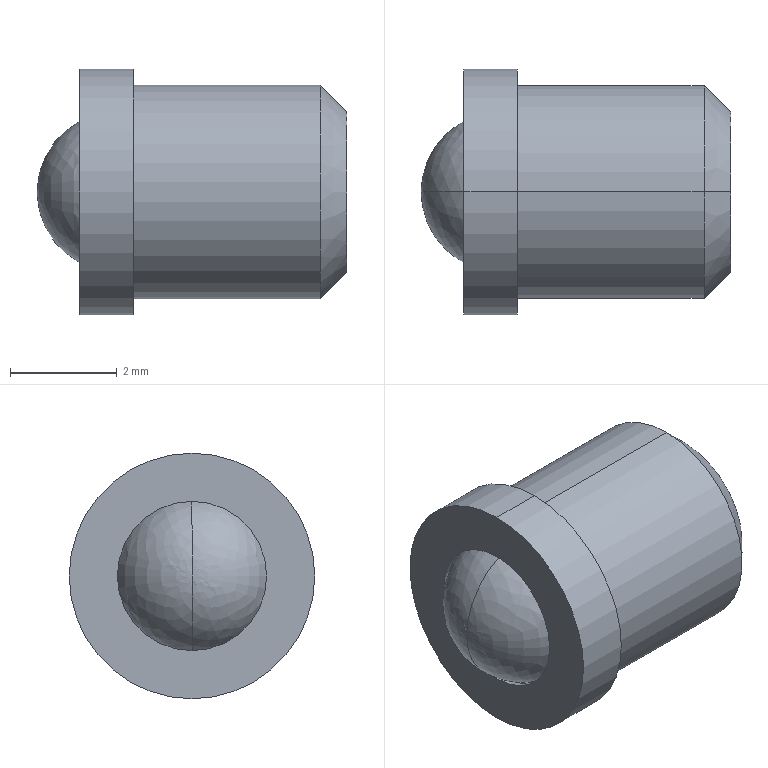Part | SolidWorks | features BaseBody 1 | 1 solid | 16 faces | box 5.8 x 4.6 x 4.6 mm | volume 67.656 mm3 | cylinder 8 | plane 4 | spline 2 | cone 2 | commonest cylinder face diameters 2.8 x2 3 x2 4 x2 4.6 x2
STEP:
#1=CARTESIAN_POINT('',(484.737,37.715,65.366));
#2=VERTEX_POINT('',#1);
#3=CARTESIAN_POINT('',(486.237,37.715,63.866));
#4=VERTEX_POINT('',#3);
#5=CARTESIAN_POINT('',(484.737,37.715,65.366));
#6=CARTESIAN_POINT('',(484.737,37.715,65.266));
#7=CARTESIAN_POINT('',(484.757,37.715,65.066));
#8=CARTESIAN_POINT('',(484.846,37.715,64.777));
#9=CARTESIAN_POINT('',(484.991,37.715,64.512));
#10=CARTESIAN_POINT('',(485.186,37.715,64.282));
#11=CARTESIAN_POINT('',(485.423,37.715,64.094));
#12=CARTESIAN_POINT('',(485.692,37.715,63.958));
#13=CARTESIAN_POINT('',(485.968,37.715,63.882));
#14=CARTESIAN_POINT('',(486.152,37.715,63.866));
#15=CARTESIAN_POINT('',(486.237,37.715,63.866));
#16=B_SPLINE_CURVE_WITH_KNOTS('',3,(#5,#6,#7,#8,#9,#10,#11,#12,#13,#14,#15),.UNSPECIFIED.,.F.,.F.,(4,1,1,1,1,1,1,1,4),(0.,0.125,0.25,0.375,0.5,0.625,0.75,0.875,0.9804),.UNSPECIFIED.);
#17=EDGE_CURVE('',#2,#4,#16,.T.);
#18=ORIENTED_EDGE('',*,*,#17,.F.);
#19=CARTESIAN_POINT('',(486.237,37.715,66.866));
#20=VERTEX_POINT('',#19);
#21=CARTESIAN_POINT('',(484.737,37.715,65.366));
#22=CARTESIAN_POINT('',(484.737,37.715,65.466));
#23=CARTESIAN_POINT('',(484.757,37.715,65.666));
#24=CARTESIAN_POINT('',(484.846,37.715,65.955));
#25=CARTESIAN_POINT('',(484.991,37.715,66.22));
#26=CARTESIAN_POINT('',(485.186,37.715,66.45));
#27=CARTESIAN_POINT('',(485.423,37.715,66.638));
#28=CARTESIAN_POINT('',(485.692,37.715,66.774));
#29=CARTESIAN_POINT('',(485.968,37.715,66.85));
#30=CARTESIAN_POINT('',(486.152,37.715,66.866));
#31=CARTESIAN_POINT('',(486.237,37.715,66.866));
#32=B_SPLINE_CURVE_WITH_KNOTS('',3,(#21,#22,#23,#24,#25,#26,#27,#28,#29,#30,#31),.UNSPECIFIED.,.F.,.F.,(4,1,1,1,1,1,1,1,4),(0.,0.125,0.25,0.375,0.5,0.625,0.75,0.875,0.9804),.UNSPECIFIED.);
#33=EDGE_CURVE('',#2,#20,#32,.T.);
#34=ORIENTED_EDGE('',*,*,#33,.T.);
#35=CARTESIAN_POINT('',(486.237,37.715,65.366));
#36=DIRECTION('',(1.,0.,0.000000013));
#37=DIRECTION('',(0.000000013,0.,-1.));
#38=AXIS2_PLACEMENT_3D('',#35,#36,#37);
#39=CIRCLE('',#38,1.5);
#40=EDGE_CURVE('',#4,#20,#39,.T.);
#41=ORIENTED_EDGE('',*,*,#40,.F.);
#42=EDGE_LOOP('',(#18,#34,#41));
#43=FACE_OUTER_BOUND('',#42,.T.);
#44=CARTESIAN_POINT('',(484.737,37.715,65.366));
#45=CARTESIAN_POINT('',(484.737,37.715,65.366));
#46=CARTESIAN_POINT('',(484.737,37.715,65.366));
#47=CARTESIAN_POINT('',(484.737,37.715,65.366));
#48=CARTESIAN_POINT('',(484.737,37.715,65.266));
#49=CARTESIAN_POINT('',(484.737,37.915,65.266));
#50=CARTESIAN_POINT('',(484.737,37.915,65.466));
#51=CARTESIAN_POINT('',(484.737,37.715,65.466));
#52=CARTESIAN_POINT('',(484.757,37.715,65.066));
#53=CARTESIAN_POINT('',(484.757,38.316,65.066));
#54=CARTESIAN_POINT('',(484.757,38.316,65.666));
#55=CARTESIAN_POINT('',(484.757,37.715,65.666));
#56=CARTESIAN_POINT('',(484.846,37.715,64.777));
#57=CARTESIAN_POINT('',(484.846,38.892,64.777));
#58=CARTESIAN_POINT('',(484.846,38.892,65.955));
#59=CARTESIAN_POINT('',(484.846,37.715,65.955));
#60=CARTESIAN_POINT('',(484.991,37.715,64.512));
#61=CARTESIAN_POINT('',(484.991,39.422,64.512));
#62=CARTESIAN_POINT('',(484.991,39.422,66.22));
#63=CARTESIAN_POINT('',(484.991,37.715,66.22));
#64=CARTESIAN_POINT('',(485.186,37.715,64.282));
#65=CARTESIAN_POINT('',(485.186,39.884,64.282));
#66=CARTESIAN_POINT('',(485.186,39.884,66.45));
#67=CARTESIAN_POINT('',(485.186,37.715,66.45));
#68=CARTESIAN_POINT('',(485.423,37.715,64.094));
#69=CARTESIAN_POINT('',(485.423,40.258,64.094));
#70=CARTESIAN_POINT('',(485.423,40.258,66.638));
#71=CARTESIAN_POINT('',(485.423,37.715,66.638));
#72=CARTESIAN_POINT('',(485.692,37.715,63.958));
#73=CARTESIAN_POINT('',(485.692,40.531,63.958));
#74=CARTESIAN_POINT('',(485.692,40.531,66.774));
#75=CARTESIAN_POINT('',(485.692,37.715,66.774));
#76=CARTESIAN_POINT('',(485.968,37.715,63.882));
#77=CARTESIAN_POINT('',(485.968,40.683,63.882));
#78=CARTESIAN_POINT('',(485.968,40.683,66.85));
#79=CARTESIAN_POINT('',(485.968,37.715,66.85));
#80=CARTESIAN_POINT('',(486.152,37.715,63.866));
#81=CARTESIAN_POINT('',(486.152,40.715,63.866));
#82=CARTESIAN_POINT('',(486.152,40.715,66.866));
#83=CARTESIAN_POINT('',(486.152,37.715,66.866));
#84=CARTESIAN_POINT('',(486.237,37.715,63.866));
#85=CARTESIAN_POINT('',(486.237,40.715,63.866));
#86=CARTESIAN_POINT('',(486.237,40.715,66.866));
#87=CARTESIAN_POINT('',(486.237,37.715,66.866));
#88=(BOUNDED_SURFACE()B_SPLINE_SURFACE(3,3,((#44,#45,#46,#47),(#48,#49,#50,#51),(#52,#53,#54,#55),(#56,#57,#58,#59),(#60,#61,#62,#63),(#64,#65,#66,#67),(#68,#69,#70,#71),(#72,#73,#74,#75),(#76,#77,#78,#79),(#80,#81,#82,#83),(#84,#85,#86,#87)),.UNSPECIFIED.,.F.,.F.,.F.)B_SPLINE_SURFACE_WITH_KNOTS((4,1,1,1,1,1,1,1,4),(4,4),(0.,0.125,0.25,0.375,0.5,0.625,0.75,0.875,0.9804),(0.,1.),.UNSPECIFIED.)GEOMETRIC_REPRESENTATION_ITEM()RATIONAL_B_SPLINE_SURFACE(((1.,0.3333,0.3333,1.),(1.,0.3333,0.3333,1.),(1.,0.3333,0.3333,1.),(1.,0.3333,0.3333,1.),(1.,0.3333,0.3333,1.),(1.,0.3333,0.3333,1.),(1.,0.3333,0.3333,1.),(1.,0.3333,0.3333,1.),(1.,0.3333,0.3333,1.),(1.,0.3333,0.3333,1.),(1.,0.3333,0.3333,1.)))REPRESENTATION_ITEM('')SURFACE());
#89=ADVANCED_FACE('',(#43),#88,.F.);
#90=CARTESIAN_POINT('',(486.537,37.715,67.366));
#91=VERTEX_POINT('',#90);
#92=CARTESIAN_POINT('',(486.537,37.715,63.366));
#93=VERTEX_POINT('',#92);
#94=CARTESIAN_POINT('',(486.537,37.715,65.366));
#95=DIRECTION('',(-1.,0.,-0.000000013));
#96=DIRECTION('',(0.000000013,0.,-1.));
#97=AXIS2_PLACEMENT_3D('',#94,#95,#96);
#98=CIRCLE('',#97,2.);
#99=EDGE_CURVE('',#91,#93,#98,.T.);
#100=ORIENTED_EDGE('',*,*,#99,.F.);
#101=CARTESIAN_POINT('',(490.037,37.715,67.366));
#102=VERTEX_POINT('',#101);
#103=CARTESIAN_POINT('',(486.537,37.715,67.366));
#104=DIRECTION('',(1.,0.,0.000000013));
#105=VECTOR('',#104,1000.);
#106=LINE('',#103,#105);
#107=EDGE_CURVE('',#91,#102,#106,.T.);
#108=ORIENTED_EDGE('',*,*,#107,.T.);
#109=CARTESIAN_POINT('',(490.037,37.715,63.366));
#110=VERTEX_POINT('',#109);
#111=CARTESIAN_POINT('',(490.037,37.715,65.366));
#112=DIRECTION('',(1.,0.,0.000000013));
#113=DIRECTION('',(0.000000013,0.,-1.));
#114=AXIS2_PLACEMENT_3D('',#111,#112,#113);
#115=CIRCLE('',#114,2.);
#116=EDGE_CURVE('',#110,#102,#115,.T.);
#117=ORIENTED_EDGE('',*,*,#116,.F.);
#118=CARTESIAN_POINT('',(486.537,37.715,63.366));
#119=DIRECTION('',(1.,0.,0.000000013));
#120=VECTOR('',#119,1000.);
#121=LINE('',#118,#120);
#122=EDGE_CURVE('',#93,#110,#121,.T.);
#123=ORIENTED_EDGE('',*,*,#122,.F.);
#124=EDGE_LOOP('',(#100,#108,#117,#123));
#125=FACE_OUTER_BOUND('',#124,.T.);
#126=CARTESIAN_POINT('',(486.537,37.715,65.366));
#127=DIRECTION('',(1.,0.,0.000000013));
#128=DIRECTION('',(0.000000013,0.,-1.));
#129=AXIS2_PLACEMENT_3D('',#126,#127,#128);
#130=CYLINDRICAL_SURFACE('',#129,2.);
#131=ADVANCED_FACE('',(#125),#130,.T.);
#132=CARTESIAN_POINT('',(490.537,37.715,63.866));
#133=VERTEX_POINT('',#132);
#134=CARTESIAN_POINT('',(490.537,37.715,66.866));
#135=VERTEX_POINT('',#134);
#136=CARTESIAN_POINT('',(490.537,37.715,65.366));
#137=DIRECTION('',(1.,0.,0.000000013));
#138=DIRECTION('',(-0.000000013,0.,1.));
#139=AXIS2_PLACEMENT_3D('',#136,#137,#138);
#140=CIRCLE('',#139,1.5);
#141=EDGE_CURVE('',#133,#135,#140,.T.);
#142=ORIENTED_EDGE('',*,*,#141,.F.);
#143=CARTESIAN_POINT('',(490.037,37.715,63.366));
#144=DIRECTION('',(-0.7071,0.,-0.7071));
#145=VECTOR('',#144,1000.);
#146=LINE('',#143,#145);
#147=EDGE_CURVE('',#133,#110,#146,.T.);
#148=ORIENTED_EDGE('',*,*,#147,.T.);
#149=ORIENTED_EDGE('',*,*,#116,.T.);
#150=CARTESIAN_POINT('',(490.037,37.715,67.366));
#151=DIRECTION('',(-0.7071,0.,0.7071));
#152=VECTOR('',#151,1000.);
#153=LINE('',#150,#152);
#154=EDGE_CURVE('',#135,#102,#153,.T.);
#155=ORIENTED_EDGE('',*,*,#154,.F.);
#156=EDGE_LOOP('',(#142,#148,#149,#155));
#157=FACE_OUTER_BOUND('',#156,.T.);
#158=CARTESIAN_POINT('',(490.037,37.715,65.366));
#159=DIRECTION('',(-1.,0.,-0.000000013));
#160=DIRECTION('',(-0.000000013,0.,1.));
#161=AXIS2_PLACEMENT_3D('',#158,#159,#160);
#162=CONICAL_SURFACE('',#161,2.,0.7854);
#163=ADVANCED_FACE('',(#157),#162,.T.);
#164=CARTESIAN_POINT('',(485.537,37.715,67.666));
#165=VERTEX_POINT('',#164);
#166=CARTESIAN_POINT('',(485.537,37.715,63.066));
#167=VERTEX_POINT('',#166);
#168=CARTESIAN_POINT('',(485.537,37.715,65.366));
#169=DIRECTION('',(-1.,0.,-0.000000013));
#170=DIRECTION('',(0.000000013,0.,-1.));
#171=AXIS2_PLACEMENT_3D('',#168,#169,#170);
#172=CIRCLE('',#171,2.3);
#173=EDGE_CURVE('',#165,#167,#172,.T.);
#174=ORIENTED_EDGE('',*,*,#173,.F.);
#175=CARTESIAN_POINT('',(486.537,37.715,67.666));
#176=VERTEX_POINT('',#175);
#177=CARTESIAN_POINT('',(485.537,37.715,67.666));
#178=DIRECTION('',(1.,0.,0.000000013));
#179=VECTOR('',#178,1000.);
#180=LINE('',#177,#179);
#181=EDGE_CURVE('',#165,#176,#180,.T.);
#182=ORIENTED_EDGE('',*,*,#181,.T.);
#183=CARTESIAN_POINT('',(486.537,37.715,63.066));
#184=VERTEX_POINT('',#183);
#185=CARTESIAN_POINT('',(486.537,37.715,65.366));
#186=DIRECTION('',(1.,0.,0.000000013));
#187=DIRECTION('',(0.000000013,0.,-1.));
#188=AXIS2_PLACEMENT_3D('',#185,#186,#187);
#189=CIRCLE('',#188,2.3);
#190=EDGE_CURVE('',#184,#176,#189,.T.);
#191=ORIENTED_EDGE('',*,*,#190,.F.);
#192=CARTESIAN_POINT('',(485.537,37.715,63.066));
#193=DIRECTION('',(1.,0.,0.000000013));
#194=VECTOR('',#193,1000.);
#195=LINE('',#192,#194);
#196=EDGE_CURVE('',#167,#184,#195,.T.);
#197=ORIENTED_EDGE('',*,*,#196,.F.);
#198=EDGE_LOOP('',(#174,#182,#191,#197));
#199=FACE_OUTER_BOUND('',#198,.T.);
#200=CARTESIAN_POINT('',(485.537,37.715,65.366));
#201=DIRECTION('',(1.,0.,0.000000013));
#202=DIRECTION('',(0.000000013,0.,-1.));
#203=AXIS2_PLACEMENT_3D('',#200,#201,#202);
#204=CYLINDRICAL_SURFACE('',#203,2.3);
#205=ADVANCED_FACE('',(#199),#204,.T.);
#206=CARTESIAN_POINT('',(485.537,37.715,63.966));
#207=VERTEX_POINT('',#206);
#208=CARTESIAN_POINT('',(485.537,37.715,66.766));
#209=VERTEX_POINT('',#208);
#210=CARTESIAN_POINT('',(485.537,37.715,65.366));
#211=DIRECTION('',(-1.,0.,-0.000000013));
#212=DIRECTION('',(0.000000013,0.,-1.));
#213=AXIS2_PLACEMENT_3D('',#210,#211,#212);
#214=CIRCLE('',#213,1.4);
#215=EDGE_CURVE('',#207,#209,#214,.T.);
#216=ORIENTED_EDGE('',*,*,#215,.T.);
#217=CARTESIAN_POINT('',(485.637,37.715,66.766));
#218=VERTEX_POINT('',#217);
#219=CARTESIAN_POINT('',(485.537,37.715,66.766));
#220=DIRECTION('',(1.,0.,0.000000013));
#221=VECTOR('',#220,1000.);
#222=LINE('',#219,#221);
#223=EDGE_CURVE('',#209,#218,#222,.T.);
#224=ORIENTED_EDGE('',*,*,#223,.T.);
#225=CARTESIAN_POINT('',(485.637,37.715,63.966));
#226=VERTEX_POINT('',#225);
#227=CARTESIAN_POINT('',(485.637,37.715,65.366));
#228=DIRECTION('',(1.,0.,0.000000013));
#229=DIRECTION('',(0.000000013,0.,-1.));
#230=AXIS2_PLACEMENT_3D('',#227,#228,#229);
#231=CIRCLE('',#230,1.4);
#232=EDGE_CURVE('',#218,#226,#231,.T.);
#233=ORIENTED_EDGE('',*,*,#232,.T.);
#234=CARTESIAN_POINT('',(485.537,37.715,63.966));
#235=DIRECTION('',(1.,0.,0.000000013));
#236=VECTOR('',#235,1000.);
#237=LINE('',#234,#236);
#238=EDGE_CURVE('',#207,#226,#237,.T.);
#239=ORIENTED_EDGE('',*,*,#238,.F.);
#240=EDGE_LOOP('',(#216,#224,#233,#239));
#241=FACE_OUTER_BOUND('',#240,.T.);
#242=CARTESIAN_POINT('',(485.537,37.715,65.366));
#243=DIRECTION('',(1.,0.,0.000000013));
#244=DIRECTION('',(0.000000013,0.,-1.));
#245=AXIS2_PLACEMENT_3D('',#242,#243,#244);
#246=CYLINDRICAL_SURFACE('',#245,1.4);
#247=ADVANCED_FACE('',(#241),#246,.F.);
#248=CARTESIAN_POINT('',(485.637,37.715,66.866));
#249=VERTEX_POINT('',#248);
#250=CARTESIAN_POINT('',(485.637,37.715,63.866));
#251=VERTEX_POINT('',#250);
#252=CARTESIAN_POINT('',(485.637,37.715,65.366));
#253=DIRECTION('',(1.,0.,0.000000013));
#254=DIRECTION('',(0.000000013,0.,-1.));
#255=AXIS2_PLACEMENT_3D('',#252,#253,#254);
#256=CIRCLE('',#255,1.5);
#257=EDGE_CURVE('',#249,#251,#256,.T.);
#258=ORIENTED_EDGE('',*,*,#257,.F.);
#259=CARTESIAN_POINT('',(485.637,37.715,66.866));
#260=DIRECTION('',(1.,0.,0.000000013));
#261=VECTOR('',#260,1000.);
#262=LINE('',#259,#261);
#263=EDGE_CURVE('',#249,#20,#262,.T.);
#264=ORIENTED_EDGE('',*,*,#263,.T.);
#265=CARTESIAN_POINT('',(486.237,37.715,65.366));
#266=DIRECTION('',(1.,0.,0.000000013));
#267=DIRECTION('',(0.000000013,0.,-1.));
#268=AXIS2_PLACEMENT_3D('',#265,#266,#267);
#269=CIRCLE('',#268,1.5);
#270=EDGE_CURVE('',#20,#4,#269,.T.);
#271=ORIENTED_EDGE('',*,*,#270,.T.);
#272=CARTESIAN_POINT('',(485.637,37.715,63.866));
#273=DIRECTION('',(1.,0.,0.000000013));
#274=VECTOR('',#273,1000.);
#275=LINE('',#272,#274);
#276=EDGE_CURVE('',#251,#4,#275,.T.);
#277=ORIENTED_EDGE('',*,*,#276,.F.);
#278=EDGE_LOOP('',(#258,#264,#271,#277));
#279=FACE_OUTER_BOUND('',#278,.T.);
#280=CARTESIAN_POINT('',(485.637,37.715,65.366));
#281=DIRECTION('',(1.,0.,0.000000013));
#282=DIRECTION('',(0.000000013,0.,-1.));
#283=AXIS2_PLACEMENT_3D('',#280,#281,#282);
#284=CYLINDRICAL_SURFACE('',#283,1.5);
#285=ADVANCED_FACE('',(#279),#284,.F.);
#286=ORIENTED_EDGE('',*,*,#107,.F.);
#287=CARTESIAN_POINT('',(486.537,37.715,65.366));
#288=DIRECTION('',(-1.,0.,-0.000000013));
#289=DIRECTION('',(0.000000013,0.,-1.));
#290=AXIS2_PLACEMENT_3D('',#287,#288,#289);
#291=CIRCLE('',#290,2.);
#292=EDGE_CURVE('',#93,#91,#291,.T.);
#293=ORIENTED_EDGE('',*,*,#292,.F.);
#294=ORIENTED_EDGE('',*,*,#122,.T.);
#295=CARTESIAN_POINT('',(490.037,37.715,65.366));
#296=DIRECTION('',(1.,0.,0.000000013));
#297=DIRECTION('',(0.000000013,0.,-1.));
#298=AXIS2_PLACEMENT_3D('',#295,#296,#297);
#299=CIRCLE('',#298,2.);
#300=EDGE_CURVE('',#102,#110,#299,.T.);
#301=ORIENTED_EDGE('',*,*,#300,.F.);
#302=EDGE_LOOP('',(#286,#293,#294,#301));
#303=FACE_OUTER_BOUND('',#302,.T.);
#304=CARTESIAN_POINT('',(486.537,37.715,65.366));
#305=DIRECTION('',(1.,0.,0.000000013));
#306=DIRECTION('',(0.000000013,0.,-1.));
#307=AXIS2_PLACEMENT_3D('',#304,#305,#306);
#308=CYLINDRICAL_SURFACE('',#307,2.);
#309=ADVANCED_FACE('',(#303),#308,.T.);
#310=ORIENTED_EDGE('',*,*,#292,.T.);
#311=ORIENTED_EDGE('',*,*,#99,.T.);
#312=EDGE_LOOP('',(#310,#311));
#313=FACE_BOUND('',#312,.T.);
#314=ORIENTED_EDGE('',*,*,#190,.T.);
#315=CARTESIAN_POINT('',(486.537,37.715,65.366));
#316=DIRECTION('',(1.,0.,0.000000013));
#317=DIRECTION('',(0.000000013,0.,-1.));
#318=AXIS2_PLACEMENT_3D('',#315,#316,#317);
#319=CIRCLE('',#318,2.3);
#320=EDGE_CURVE('',#176,#184,#319,.T.);
#321=ORIENTED_EDGE('',*,*,#320,.T.);
#322=EDGE_LOOP('',(#314,#321));
#323=FACE_OUTER_BOUND('',#322,.T.);
#324=CARTESIAN_POINT('',(486.537,35.323,67.758));
#325=DIRECTION('',(1.,0.,0.000000013));
#326=DIRECTION('',(0.000000013,0.,-1.));
#327=AXIS2_PLACEMENT_3D('',#324,#325,#326);
#328=PLANE('',#327);
#329=ADVANCED_FACE('',(#313,#323),#328,.T.);
#330=ORIENTED_EDGE('',*,*,#147,.F.);
#331=CARTESIAN_POINT('',(490.537,37.715,65.366));
#332=DIRECTION('',(1.,0.,0.000000013));
#333=DIRECTION('',(-0.000000013,0.,1.));
#334=AXIS2_PLACEMENT_3D('',#331,#332,#333);
#335=CIRCLE('',#334,1.5);
#336=EDGE_CURVE('',#135,#133,#335,.T.);
#337=ORIENTED_EDGE('',*,*,#336,.F.);
#338=ORIENTED_EDGE('',*,*,#154,.T.);
#339=ORIENTED_EDGE('',*,*,#300,.T.);
#340=EDGE_LOOP('',(#330,#337,#338,#339));
#341=FACE_OUTER_BOUND('',#340,.T.);
#342=CARTESIAN_POINT('',(490.037,37.715,65.366));
#343=DIRECTION('',(-1.,0.,-0.000000013));
#344=DIRECTION('',(-0.000000013,0.,1.));
#345=AXIS2_PLACEMENT_3D('',#342,#343,#344);
#346=CONICAL_SURFACE('',#345,2.,0.7854);
#347=ADVANCED_FACE('',(#341),#346,.T.);
#348=ORIENTED_EDGE('',*,*,#181,.F.);
#349=CARTESIAN_POINT('',(485.537,37.715,65.366));
#350=DIRECTION('',(-1.,0.,-0.000000013));
#351=DIRECTION('',(0.000000013,0.,-1.));
#352=AXIS2_PLACEMENT_3D('',#349,#350,#351);
#353=CIRCLE('',#352,2.3);
#354=EDGE_CURVE('',#167,#165,#353,.T.);
#355=ORIENTED_EDGE('',*,*,#354,.F.);
#356=ORIENTED_EDGE('',*,*,#196,.T.);
#357=ORIENTED_EDGE('',*,*,#320,.F.);
#358=EDGE_LOOP('',(#348,#355,#356,#357));
#359=FACE_OUTER_BOUND('',#358,.T.);
#360=CARTESIAN_POINT('',(485.537,37.715,65.366));
#361=DIRECTION('',(1.,0.,0.000000013));
#362=DIRECTION('',(0.000000013,0.,-1.));
#363=AXIS2_PLACEMENT_3D('',#360,#361,#362);
#364=CYLINDRICAL_SURFACE('',#363,2.3);
#365=ADVANCED_FACE('',(#359),#364,.T.);
#366=ORIENTED_EDGE('',*,*,#336,.T.);
#367=ORIENTED_EDGE('',*,*,#141,.T.);
#368=EDGE_LOOP('',(#366,#367));
#369=FACE_OUTER_BOUND('',#368,.T.);
#370=CARTESIAN_POINT('',(490.537,36.155,66.926));
#371=DIRECTION('',(1.,0.,0.000000013));
#372=DIRECTION('',(0.000000013,0.,-1.));
#373=AXIS2_PLACEMENT_3D('',#370,#371,#372);
#374=PLANE('',#373);
#375=ADVANCED_FACE('',(#369),#374,.T.);
#376=ORIENTED_EDGE('',*,*,#215,.F.);
#377=CARTESIAN_POINT('',(485.537,37.715,65.366));
#378=DIRECTION('',(-1.,0.,-0.000000013));
#379=DIRECTION('',(0.000000013,0.,-1.));
#380=AXIS2_PLACEMENT_3D('',#377,#378,#379);
#381=CIRCLE('',#380,1.4);
#382=EDGE_CURVE('',#209,#207,#381,.T.);
#383=ORIENTED_EDGE('',*,*,#382,.F.);
#384=EDGE_LOOP('',(#376,#383));
#385=FACE_BOUND('',#384,.T.);
#386=ORIENTED_EDGE('',*,*,#354,.T.);
#387=ORIENTED_EDGE('',*,*,#173,.T.);
#388=EDGE_LOOP('',(#386,#387));
#389=FACE_OUTER_BOUND('',#388,.T.);
#390=CARTESIAN_POINT('',(485.537,35.323,67.758));
#391=DIRECTION('',(1.,0.,0.000000013));
#392=DIRECTION('',(0.000000013,0.,-1.));
#393=AXIS2_PLACEMENT_3D('',#390,#391,#392);
#394=PLANE('',#393);
#395=ADVANCED_FACE('',(#385,#389),#394,.F.);
#396=ORIENTED_EDGE('',*,*,#223,.F.);
#397=ORIENTED_EDGE('',*,*,#382,.T.);
#398=ORIENTED_EDGE('',*,*,#238,.T.);
#399=CARTESIAN_POINT('',(485.637,37.715,65.366));
#400=DIRECTION('',(1.,0.,0.000000013));
#401=DIRECTION('',(0.000000013,0.,-1.));
#402=AXIS2_PLACEMENT_3D('',#399,#400,#401);
#403=CIRCLE('',#402,1.4);
#404=EDGE_CURVE('',#226,#218,#403,.T.);
#405=ORIENTED_EDGE('',*,*,#404,.T.);
#406=EDGE_LOOP('',(#396,#397,#398,#405));
#407=FACE_OUTER_BOUND('',#406,.T.);
#408=CARTESIAN_POINT('',(485.537,37.715,65.366));
#409=DIRECTION('',(1.,0.,0.000000013));
#410=DIRECTION('',(0.000000013,0.,-1.));
#411=AXIS2_PLACEMENT_3D('',#408,#409,#410);
#412=CYLINDRICAL_SURFACE('',#411,1.4);
#413=ADVANCED_FACE('',(#407),#412,.F.);
#414=ORIENTED_EDGE('',*,*,#404,.F.);
#415=ORIENTED_EDGE('',*,*,#232,.F.);
#416=EDGE_LOOP('',(#414,#415));
#417=FACE_BOUND('',#416,.T.);
#418=CARTESIAN_POINT('',(485.637,37.715,65.366));
#419=DIRECTION('',(1.,0.,0.000000013));
#420=DIRECTION('',(0.000000013,0.,-1.));
#421=AXIS2_PLACEMENT_3D('',#418,#419,#420);
#422=CIRCLE('',#421,1.5);
#423=EDGE_CURVE('',#251,#249,#422,.T.);
#424=ORIENTED_EDGE('',*,*,#423,.T.);
#425=ORIENTED_EDGE('',*,*,#257,.T.);
#426=EDGE_LOOP('',(#424,#425));
#427=FACE_OUTER_BOUND('',#426,.T.);
#428=CARTESIAN_POINT('',(485.637,36.155,66.926));
#429=DIRECTION('',(1.,0.,0.000000013));
#430=DIRECTION('',(0.000000013,0.,-1.));
#431=AXIS2_PLACEMENT_3D('',#428,#429,#430);
#432=PLANE('',#431);
#433=ADVANCED_FACE('',(#417,#427),#432,.T.);
#434=ORIENTED_EDGE('',*,*,#263,.F.);
#435=ORIENTED_EDGE('',*,*,#423,.F.);
#436=ORIENTED_EDGE('',*,*,#276,.T.);
#437=ORIENTED_EDGE('',*,*,#40,.T.);
#438=EDGE_LOOP('',(#434,#435,#436,#437));
#439=FACE_OUTER_BOUND('',#438,.T.);
#440=CARTESIAN_POINT('',(485.637,37.715,65.366));
#441=DIRECTION('',(1.,0.,0.000000013));
#442=DIRECTION('',(0.000000013,0.,-1.));
#443=AXIS2_PLACEMENT_3D('',#440,#441,#442);
#444=CYLINDRICAL_SURFACE('',#443,1.5);
#445=ADVANCED_FACE('',(#439),#444,.F.);
#446=ORIENTED_EDGE('',*,*,#33,.F.);
#447=ORIENTED_EDGE('',*,*,#17,.T.);
#448=ORIENTED_EDGE('',*,*,#270,.F.);
#449=EDGE_LOOP('',(#446,#447,#448));
#450=FACE_OUTER_BOUND('',#449,.T.);
#451=CARTESIAN_POINT('',(484.737,37.715,65.366));
#452=CARTESIAN_POINT('',(484.737,37.715,65.366));
#453=CARTESIAN_POINT('',(484.737,37.715,65.366));
#454=CARTESIAN_POINT('',(484.737,37.715,65.366));
#455=CARTESIAN_POINT('',(484.737,37.715,65.466));
#456=CARTESIAN_POINT('',(484.737,37.514,65.466));
#457=CARTESIAN_POINT('',(484.737,37.514,65.266));
#458=CARTESIAN_POINT('',(484.737,37.715,65.266));
#459=CARTESIAN_POINT('',(484.757,37.715,65.666));
#460=CARTESIAN_POINT('',(484.757,37.114,65.666));
#461=CARTESIAN_POINT('',(484.757,37.114,65.066));
#462=CARTESIAN_POINT('',(484.757,37.715,65.066));
#463=CARTESIAN_POINT('',(484.846,37.715,65.955));
#464=CARTESIAN_POINT('',(484.846,36.537,65.955));
#465=CARTESIAN_POINT('',(484.846,36.537,64.777));
#466=CARTESIAN_POINT('',(484.846,37.715,64.777));
#467=CARTESIAN_POINT('',(484.991,37.715,66.22));
#468=CARTESIAN_POINT('',(484.991,36.007,66.22));
#469=CARTESIAN_POINT('',(484.991,36.007,64.512));
#470=CARTESIAN_POINT('',(484.991,37.715,64.512));
#471=CARTESIAN_POINT('',(485.186,37.715,66.45));
#472=CARTESIAN_POINT('',(485.186,35.546,66.45));
#473=CARTESIAN_POINT('',(485.186,35.546,64.282));
#474=CARTESIAN_POINT('',(485.186,37.715,64.282));
#475=CARTESIAN_POINT('',(485.423,37.715,66.638));
#476=CARTESIAN_POINT('',(485.423,35.171,66.638));
#477=CARTESIAN_POINT('',(485.423,35.171,64.094));
#478=CARTESIAN_POINT('',(485.423,37.715,64.094));
#479=CARTESIAN_POINT('',(485.692,37.715,66.774));
#480=CARTESIAN_POINT('',(485.692,34.898,66.774));
#481=CARTESIAN_POINT('',(485.692,34.898,63.958));
#482=CARTESIAN_POINT('',(485.692,37.715,63.958));
#483=CARTESIAN_POINT('',(485.968,37.715,66.85));
#484=CARTESIAN_POINT('',(485.968,34.746,66.85));
#485=CARTESIAN_POINT('',(485.968,34.746,63.882));
#486=CARTESIAN_POINT('',(485.968,37.715,63.882));
#487=CARTESIAN_POINT('',(486.152,37.715,66.866));
#488=CARTESIAN_POINT('',(486.152,34.715,66.866));
#489=CARTESIAN_POINT('',(486.152,34.715,63.866));
#490=CARTESIAN_POINT('',(486.152,37.715,63.866));
#491=CARTESIAN_POINT('',(486.237,37.715,66.866));
#492=CARTESIAN_POINT('',(486.237,34.715,66.866));
#493=CARTESIAN_POINT('',(486.237,34.715,63.866));
#494=CARTESIAN_POINT('',(486.237,37.715,63.866));
#495=(BOUNDED_SURFACE()B_SPLINE_SURFACE(3,3,((#451,#452,#453,#454),(#455,#456,#457,#458),(#459,#460,#461,#462),(#463,#464,#465,#466),(#467,#468,#469,#470),(#471,#472,#473,#474),(#475,#476,#477,#478),(#479,#480,#481,#482),(#483,#484,#485,#486),(#487,#488,#489,#490),(#491,#492,#493,#494)),.UNSPECIFIED.,.F.,.F.,.F.)B_SPLINE_SURFACE_WITH_KNOTS((4,1,1,1,1,1,1,1,4),(4,4),(0.,0.125,0.25,0.375,0.5,0.625,0.75,0.875,0.9804),(0.,1.),.UNSPECIFIED.)GEOMETRIC_REPRESENTATION_ITEM()RATIONAL_B_SPLINE_SURFACE(((1.,0.3333,0.3333,1.),(1.,0.3333,0.3333,1.),(1.,0.3333,0.3333,1.),(1.,0.3333,0.3333,1.),(1.,0.3333,0.3333,1.),(1.,0.3333,0.3333,1.),(1.,0.3333,0.3333,1.),(1.,0.3333,0.3333,1.),(1.,0.3333,0.3333,1.),(1.,0.3333,0.3333,1.),(1.,0.3333,0.3333,1.)))REPRESENTATION_ITEM('')SURFACE());
#496=ADVANCED_FACE('',(#450),#495,.F.);
#497=CLOSED_SHELL('',(#89,#131,#163,#205,#247,#285,#309,#329,#347,#365,#375,#395,#413,#433,#445,#496));
#498=MANIFOLD_SOLID_BREP('',#497);
#499=CARTESIAN_POINT('',(0.,0.,0.));
#500=DIRECTION('',(0.,0.,1.));
#501=DIRECTION('',(1.,0.,0.));
#502=AXIS2_PLACEMENT_3D('',#499,#500,#501);
#503=(LENGTH_UNIT()NAMED_UNIT(*)SI_UNIT(.MILLI.,.METRE.));
#504=UNCERTAINTY_MEASURE_WITH_UNIT(LENGTH_MEASURE(0.00001),#503,'','');
#505=(NAMED_UNIT(*)PLANE_ANGLE_UNIT()SI_UNIT($,.RADIAN.));
#506=(NAMED_UNIT(*)SI_UNIT($,.STERADIAN.)SOLID_ANGLE_UNIT());
#507=(GEOMETRIC_REPRESENTATION_CONTEXT(3)GLOBAL_UNCERTAINTY_ASSIGNED_CONTEXT((#504))GLOBAL_UNIT_ASSIGNED_CONTEXT((#503,#505,#506))REPRESENTATION_CONTEXT('',''));
#508=ADVANCED_BREP_SHAPE_REPRESENTATION('',(#498,#502),#507);